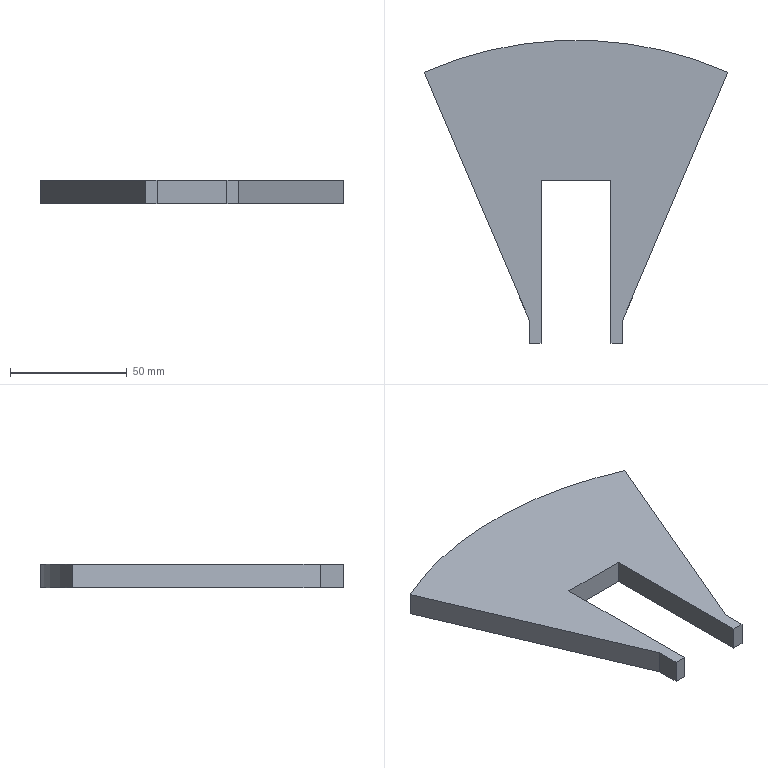Part | SolidWorks | features Extrusion 1 | 1 solid | 12 faces | box 130.202 x 130 x 10 mm | volume 85461 mm3 | plane 11 | cylinder 1 | commonest cylinder face diameters 322 x1
STEP:
#1=CARTESIAN_POINT('',(20.,41.,-5.));
#2=VERTEX_POINT('',#1);
#3=CARTESIAN_POINT('',(65.101,147.251,-5.));
#4=VERTEX_POINT('',#3);
#5=CARTESIAN_POINT('',(2.2,-0.9339,-5.));
#6=DIRECTION('',(0.3907,0.9205,0.));
#7=VECTOR('',#6,1000.);
#8=LINE('',#5,#7);
#9=EDGE_CURVE('',#2,#4,#8,.T.);
#10=ORIENTED_EDGE('',*,*,#9,.T.);
#11=CARTESIAN_POINT('',(65.101,147.251,5.));
#12=VERTEX_POINT('',#11);
#13=CARTESIAN_POINT('',(65.101,147.251,5.));
#14=DIRECTION('',(0.,0.,-1.));
#15=VECTOR('',#14,1000.);
#16=LINE('',#13,#15);
#17=EDGE_CURVE('',#12,#4,#16,.T.);
#18=ORIENTED_EDGE('',*,*,#17,.F.);
#19=CARTESIAN_POINT('',(20.,41.,5.));
#20=VERTEX_POINT('',#19);
#21=CARTESIAN_POINT('',(2.2,-0.9339,5.));
#22=DIRECTION('',(0.3907,0.9205,0.));
#23=VECTOR('',#22,1000.);
#24=LINE('',#21,#23);
#25=EDGE_CURVE('',#20,#12,#24,.T.);
#26=ORIENTED_EDGE('',*,*,#25,.F.);
#27=CARTESIAN_POINT('',(20.,41.,5.));
#28=DIRECTION('',(0.,0.,-1.));
#29=VECTOR('',#28,1000.);
#30=LINE('',#27,#29);
#31=EDGE_CURVE('',#20,#2,#30,.T.);
#32=ORIENTED_EDGE('',*,*,#31,.T.);
#33=EDGE_LOOP('',(#10,#18,#26,#32));
#34=FACE_OUTER_BOUND('',#33,.T.);
#35=CARTESIAN_POINT('',(2.2,-0.9339,5.));
#36=DIRECTION('',(-0.9205,0.3907,0.));
#37=DIRECTION('',(-0.3907,-0.9205,0.));
#38=AXIS2_PLACEMENT_3D('',#35,#36,#37);
#39=PLANE('',#38);
#40=ADVANCED_FACE('',(#34),#39,.F.);
#41=CARTESIAN_POINT('',(-65.101,147.251,-5.));
#42=VERTEX_POINT('',#41);
#43=CARTESIAN_POINT('',(0.,0.,-5.));
#44=DIRECTION('',(0.,0.,1.));
#45=DIRECTION('',(1.,0.,0.));
#46=AXIS2_PLACEMENT_3D('',#43,#44,#45);
#47=CIRCLE('',#46,161.);
#48=EDGE_CURVE('',#4,#42,#47,.T.);
#49=ORIENTED_EDGE('',*,*,#48,.T.);
#50=CARTESIAN_POINT('',(-65.101,147.251,5.));
#51=VERTEX_POINT('',#50);
#52=CARTESIAN_POINT('',(-65.101,147.251,5.));
#53=DIRECTION('',(0.,0.,-1.));
#54=VECTOR('',#53,1000.);
#55=LINE('',#52,#54);
#56=EDGE_CURVE('',#51,#42,#55,.T.);
#57=ORIENTED_EDGE('',*,*,#56,.F.);
#58=CARTESIAN_POINT('',(0.,0.,5.));
#59=DIRECTION('',(0.,0.,1.));
#60=DIRECTION('',(1.,0.,0.));
#61=AXIS2_PLACEMENT_3D('',#58,#59,#60);
#62=CIRCLE('',#61,161.);
#63=EDGE_CURVE('',#12,#51,#62,.T.);
#64=ORIENTED_EDGE('',*,*,#63,.F.);
#65=ORIENTED_EDGE('',*,*,#17,.T.);
#66=EDGE_LOOP('',(#49,#57,#64,#65));
#67=FACE_OUTER_BOUND('',#66,.T.);
#68=CARTESIAN_POINT('',(0.,0.,5.));
#69=DIRECTION('',(0.,0.,-1.));
#70=DIRECTION('',(-1.,0.,0.));
#71=AXIS2_PLACEMENT_3D('',#68,#69,#70);
#72=CYLINDRICAL_SURFACE('',#71,161.);
#73=ADVANCED_FACE('',(#67),#72,.T.);
#74=CARTESIAN_POINT('',(-20.,41.,-5.));
#75=VERTEX_POINT('',#74);
#76=CARTESIAN_POINT('',(-2.2,-0.9339,-5.));
#77=DIRECTION('',(0.3907,-0.9205,0.));
#78=VECTOR('',#77,1000.);
#79=LINE('',#76,#78);
#80=EDGE_CURVE('',#42,#75,#79,.T.);
#81=ORIENTED_EDGE('',*,*,#80,.T.);
#82=CARTESIAN_POINT('',(-20.,41.,5.));
#83=VERTEX_POINT('',#82);
#84=CARTESIAN_POINT('',(-20.,41.,5.));
#85=DIRECTION('',(0.,0.,-1.));
#86=VECTOR('',#85,1000.);
#87=LINE('',#84,#86);
#88=EDGE_CURVE('',#83,#75,#87,.T.);
#89=ORIENTED_EDGE('',*,*,#88,.F.);
#90=CARTESIAN_POINT('',(-2.2,-0.9339,5.));
#91=DIRECTION('',(0.3907,-0.9205,0.));
#92=VECTOR('',#91,1000.);
#93=LINE('',#90,#92);
#94=EDGE_CURVE('',#51,#83,#93,.T.);
#95=ORIENTED_EDGE('',*,*,#94,.F.);
#96=ORIENTED_EDGE('',*,*,#56,.T.);
#97=EDGE_LOOP('',(#81,#89,#95,#96));
#98=FACE_OUTER_BOUND('',#97,.T.);
#99=CARTESIAN_POINT('',(-2.2,-0.9339,5.));
#100=DIRECTION('',(0.9205,0.3907,0.));
#101=DIRECTION('',(-0.3907,0.9205,0.));
#102=AXIS2_PLACEMENT_3D('',#99,#100,#101);
#103=PLANE('',#102);
#104=ADVANCED_FACE('',(#98),#103,.F.);
#105=CARTESIAN_POINT('',(-20.,31.,-5.));
#106=VERTEX_POINT('',#105);
#107=CARTESIAN_POINT('',(-20.,0.,-5.));
#108=DIRECTION('',(0.,-1.,0.));
#109=VECTOR('',#108,1000.);
#110=LINE('',#107,#109);
#111=EDGE_CURVE('',#75,#106,#110,.T.);
#112=ORIENTED_EDGE('',*,*,#111,.T.);
#113=CARTESIAN_POINT('',(-20.,31.,5.));
#114=VERTEX_POINT('',#113);
#115=CARTESIAN_POINT('',(-20.,31.,5.));
#116=DIRECTION('',(0.,0.,-1.));
#117=VECTOR('',#116,1000.);
#118=LINE('',#115,#117);
#119=EDGE_CURVE('',#114,#106,#118,.T.);
#120=ORIENTED_EDGE('',*,*,#119,.F.);
#121=CARTESIAN_POINT('',(-20.,0.,5.));
#122=DIRECTION('',(0.,-1.,0.));
#123=VECTOR('',#122,1000.);
#124=LINE('',#121,#123);
#125=EDGE_CURVE('',#83,#114,#124,.T.);
#126=ORIENTED_EDGE('',*,*,#125,.F.);
#127=ORIENTED_EDGE('',*,*,#88,.T.);
#128=EDGE_LOOP('',(#112,#120,#126,#127));
#129=FACE_OUTER_BOUND('',#128,.T.);
#130=CARTESIAN_POINT('',(-20.,0.,5.));
#131=DIRECTION('',(1.,0.,0.));
#132=DIRECTION('',(0.,1.,0.));
#133=AXIS2_PLACEMENT_3D('',#130,#131,#132);
#134=PLANE('',#133);
#135=ADVANCED_FACE('',(#129),#134,.F.);
#136=CARTESIAN_POINT('',(-15.,31.,-5.));
#137=VERTEX_POINT('',#136);
#138=CARTESIAN_POINT('',(0.,31.,-5.));
#139=DIRECTION('',(1.,0.,0.));
#140=VECTOR('',#139,1000.);
#141=LINE('',#138,#140);
#142=EDGE_CURVE('',#106,#137,#141,.T.);
#143=ORIENTED_EDGE('',*,*,#142,.T.);
#144=CARTESIAN_POINT('',(-15.,31.,5.));
#145=VERTEX_POINT('',#144);
#146=CARTESIAN_POINT('',(-15.,31.,5.));
#147=DIRECTION('',(0.,0.,-1.));
#148=VECTOR('',#147,1000.);
#149=LINE('',#146,#148);
#150=EDGE_CURVE('',#145,#137,#149,.T.);
#151=ORIENTED_EDGE('',*,*,#150,.F.);
#152=CARTESIAN_POINT('',(0.,31.,5.));
#153=DIRECTION('',(1.,0.,0.));
#154=VECTOR('',#153,1000.);
#155=LINE('',#152,#154);
#156=EDGE_CURVE('',#114,#145,#155,.T.);
#157=ORIENTED_EDGE('',*,*,#156,.F.);
#158=ORIENTED_EDGE('',*,*,#119,.T.);
#159=EDGE_LOOP('',(#143,#151,#157,#158));
#160=FACE_OUTER_BOUND('',#159,.T.);
#161=CARTESIAN_POINT('',(0.,31.,5.));
#162=DIRECTION('',(0.,1.,0.));
#163=DIRECTION('',(-1.,0.,0.));
#164=AXIS2_PLACEMENT_3D('',#161,#162,#163);
#165=PLANE('',#164);
#166=ADVANCED_FACE('',(#160),#165,.F.);
#167=CARTESIAN_POINT('',(-15.,101.,-5.));
#168=VERTEX_POINT('',#167);
#169=CARTESIAN_POINT('',(-15.,0.,-5.));
#170=DIRECTION('',(0.,1.,0.));
#171=VECTOR('',#170,1000.);
#172=LINE('',#169,#171);
#173=EDGE_CURVE('',#137,#168,#172,.T.);
#174=ORIENTED_EDGE('',*,*,#173,.T.);
#175=CARTESIAN_POINT('',(-15.,101.,5.));
#176=VERTEX_POINT('',#175);
#177=CARTESIAN_POINT('',(-15.,101.,5.));
#178=DIRECTION('',(0.,0.,-1.));
#179=VECTOR('',#178,1000.);
#180=LINE('',#177,#179);
#181=EDGE_CURVE('',#176,#168,#180,.T.);
#182=ORIENTED_EDGE('',*,*,#181,.F.);
#183=CARTESIAN_POINT('',(-15.,0.,5.));
#184=DIRECTION('',(0.,1.,0.));
#185=VECTOR('',#184,1000.);
#186=LINE('',#183,#185);
#187=EDGE_CURVE('',#145,#176,#186,.T.);
#188=ORIENTED_EDGE('',*,*,#187,.F.);
#189=ORIENTED_EDGE('',*,*,#150,.T.);
#190=EDGE_LOOP('',(#174,#182,#188,#189));
#191=FACE_OUTER_BOUND('',#190,.T.);
#192=CARTESIAN_POINT('',(-15.,0.,5.));
#193=DIRECTION('',(-1.,0.,0.));
#194=DIRECTION('',(0.,0.,1.));
#195=AXIS2_PLACEMENT_3D('',#192,#193,#194);
#196=PLANE('',#195);
#197=ADVANCED_FACE('',(#191),#196,.F.);
#198=CARTESIAN_POINT('',(15.,101.,-5.));
#199=VERTEX_POINT('',#198);
#200=CARTESIAN_POINT('',(0.,101.,-5.));
#201=DIRECTION('',(-1.,0.,0.));
#202=VECTOR('',#201,1000.);
#203=LINE('',#200,#202);
#204=EDGE_CURVE('',#199,#168,#203,.T.);
#205=ORIENTED_EDGE('',*,*,#204,.F.);
#206=CARTESIAN_POINT('',(15.,101.,5.));
#207=VERTEX_POINT('',#206);
#208=CARTESIAN_POINT('',(15.,101.,5.));
#209=DIRECTION('',(0.,0.,-1.));
#210=VECTOR('',#209,1000.);
#211=LINE('',#208,#210);
#212=EDGE_CURVE('',#207,#199,#211,.T.);
#213=ORIENTED_EDGE('',*,*,#212,.F.);
#214=CARTESIAN_POINT('',(0.,101.,5.));
#215=DIRECTION('',(-1.,0.,0.));
#216=VECTOR('',#215,1000.);
#217=LINE('',#214,#216);
#218=EDGE_CURVE('',#207,#176,#217,.T.);
#219=ORIENTED_EDGE('',*,*,#218,.T.);
#220=ORIENTED_EDGE('',*,*,#181,.T.);
#221=EDGE_LOOP('',(#205,#213,#219,#220));
#222=FACE_OUTER_BOUND('',#221,.T.);
#223=CARTESIAN_POINT('',(0.,101.,5.));
#224=DIRECTION('',(0.,-1.,0.));
#225=DIRECTION('',(0.,0.,-1.));
#226=AXIS2_PLACEMENT_3D('',#223,#224,#225);
#227=PLANE('',#226);
#228=ADVANCED_FACE('',(#222),#227,.T.);
#229=CARTESIAN_POINT('',(15.,31.,-5.));
#230=VERTEX_POINT('',#229);
#231=CARTESIAN_POINT('',(15.,0.,-5.));
#232=DIRECTION('',(0.,1.,0.));
#233=VECTOR('',#232,1000.);
#234=LINE('',#231,#233);
#235=EDGE_CURVE('',#230,#199,#234,.T.);
#236=ORIENTED_EDGE('',*,*,#235,.F.);
#237=CARTESIAN_POINT('',(15.,31.,5.));
#238=VERTEX_POINT('',#237);
#239=CARTESIAN_POINT('',(15.,31.,5.));
#240=DIRECTION('',(0.,0.,-1.));
#241=VECTOR('',#240,1000.);
#242=LINE('',#239,#241);
#243=EDGE_CURVE('',#238,#230,#242,.T.);
#244=ORIENTED_EDGE('',*,*,#243,.F.);
#245=CARTESIAN_POINT('',(15.,0.,5.));
#246=DIRECTION('',(0.,1.,0.));
#247=VECTOR('',#246,1000.);
#248=LINE('',#245,#247);
#249=EDGE_CURVE('',#238,#207,#248,.T.);
#250=ORIENTED_EDGE('',*,*,#249,.T.);
#251=ORIENTED_EDGE('',*,*,#212,.T.);
#252=EDGE_LOOP('',(#236,#244,#250,#251));
#253=FACE_OUTER_BOUND('',#252,.T.);
#254=CARTESIAN_POINT('',(15.,0.,5.));
#255=DIRECTION('',(-1.,0.,0.));
#256=DIRECTION('',(0.,-1.,0.));
#257=AXIS2_PLACEMENT_3D('',#254,#255,#256);
#258=PLANE('',#257);
#259=ADVANCED_FACE('',(#253),#258,.T.);
#260=CARTESIAN_POINT('',(20.,31.,-5.));
#261=VERTEX_POINT('',#260);
#262=CARTESIAN_POINT('',(0.,31.,-5.));
#263=DIRECTION('',(1.,0.,0.));
#264=VECTOR('',#263,1000.);
#265=LINE('',#262,#264);
#266=EDGE_CURVE('',#230,#261,#265,.T.);
#267=ORIENTED_EDGE('',*,*,#266,.T.);
#268=CARTESIAN_POINT('',(20.,31.,5.));
#269=VERTEX_POINT('',#268);
#270=CARTESIAN_POINT('',(20.,31.,5.));
#271=DIRECTION('',(0.,0.,-1.));
#272=VECTOR('',#271,1000.);
#273=LINE('',#270,#272);
#274=EDGE_CURVE('',#269,#261,#273,.T.);
#275=ORIENTED_EDGE('',*,*,#274,.F.);
#276=CARTESIAN_POINT('',(0.,31.,5.));
#277=DIRECTION('',(1.,0.,0.));
#278=VECTOR('',#277,1000.);
#279=LINE('',#276,#278);
#280=EDGE_CURVE('',#238,#269,#279,.T.);
#281=ORIENTED_EDGE('',*,*,#280,.F.);
#282=ORIENTED_EDGE('',*,*,#243,.T.);
#283=EDGE_LOOP('',(#267,#275,#281,#282));
#284=FACE_OUTER_BOUND('',#283,.T.);
#285=CARTESIAN_POINT('',(0.,31.,5.));
#286=DIRECTION('',(0.,1.,0.));
#287=DIRECTION('',(-1.,0.,0.));
#288=AXIS2_PLACEMENT_3D('',#285,#286,#287);
#289=PLANE('',#288);
#290=ADVANCED_FACE('',(#284),#289,.F.);
#291=CARTESIAN_POINT('',(20.,0.,-5.));
#292=DIRECTION('',(0.,1.,0.));
#293=VECTOR('',#292,1000.);
#294=LINE('',#291,#293);
#295=EDGE_CURVE('',#261,#2,#294,.T.);
#296=ORIENTED_EDGE('',*,*,#295,.T.);
#297=ORIENTED_EDGE('',*,*,#31,.F.);
#298=CARTESIAN_POINT('',(20.,0.,5.));
#299=DIRECTION('',(0.,1.,0.));
#300=VECTOR('',#299,1000.);
#301=LINE('',#298,#300);
#302=EDGE_CURVE('',#269,#20,#301,.T.);
#303=ORIENTED_EDGE('',*,*,#302,.F.);
#304=ORIENTED_EDGE('',*,*,#274,.T.);
#305=EDGE_LOOP('',(#296,#297,#303,#304));
#306=FACE_OUTER_BOUND('',#305,.T.);
#307=CARTESIAN_POINT('',(20.,0.,5.));
#308=DIRECTION('',(-1.,0.,0.));
#309=DIRECTION('',(0.,-1.,0.));
#310=AXIS2_PLACEMENT_3D('',#307,#308,#309);
#311=PLANE('',#310);
#312=ADVANCED_FACE('',(#306),#311,.F.);
#313=ORIENTED_EDGE('',*,*,#25,.T.);
#314=ORIENTED_EDGE('',*,*,#63,.T.);
#315=ORIENTED_EDGE('',*,*,#94,.T.);
#316=ORIENTED_EDGE('',*,*,#125,.T.);
#317=ORIENTED_EDGE('',*,*,#156,.T.);
#318=ORIENTED_EDGE('',*,*,#187,.T.);
#319=ORIENTED_EDGE('',*,*,#218,.F.);
#320=ORIENTED_EDGE('',*,*,#249,.F.);
#321=ORIENTED_EDGE('',*,*,#280,.T.);
#322=ORIENTED_EDGE('',*,*,#302,.T.);
#323=EDGE_LOOP('',(#313,#314,#315,#316,#317,#318,#319,#320,#321,#322));
#324=FACE_OUTER_BOUND('',#323,.T.);
#325=CARTESIAN_POINT('',(0.,0.,5.));
#326=DIRECTION('',(0.,0.,1.));
#327=DIRECTION('',(1.,0.,0.));
#328=AXIS2_PLACEMENT_3D('',#325,#326,#327);
#329=PLANE('',#328);
#330=ADVANCED_FACE('',(#324),#329,.T.);
#331=ORIENTED_EDGE('',*,*,#9,.F.);
#332=ORIENTED_EDGE('',*,*,#295,.F.);
#333=ORIENTED_EDGE('',*,*,#266,.F.);
#334=ORIENTED_EDGE('',*,*,#235,.T.);
#335=ORIENTED_EDGE('',*,*,#204,.T.);
#336=ORIENTED_EDGE('',*,*,#173,.F.);
#337=ORIENTED_EDGE('',*,*,#142,.F.);
#338=ORIENTED_EDGE('',*,*,#111,.F.);
#339=ORIENTED_EDGE('',*,*,#80,.F.);
#340=ORIENTED_EDGE('',*,*,#48,.F.);
#341=EDGE_LOOP('',(#331,#332,#333,#334,#335,#336,#337,#338,#339,#340));
#342=FACE_OUTER_BOUND('',#341,.T.);
#343=CARTESIAN_POINT('',(0.,0.,-5.));
#344=DIRECTION('',(0.,0.,1.));
#345=DIRECTION('',(1.,0.,0.));
#346=AXIS2_PLACEMENT_3D('',#343,#344,#345);
#347=PLANE('',#346);
#348=ADVANCED_FACE('',(#342),#347,.F.);
#349=CLOSED_SHELL('',(#40,#73,#104,#135,#166,#197,#228,#259,#290,#312,#330,#348));
#350=MANIFOLD_SOLID_BREP('',#349);
#351=CARTESIAN_POINT('',(0.,0.,0.));
#352=DIRECTION('',(0.,0.,1.));
#353=DIRECTION('',(1.,0.,0.));
#354=AXIS2_PLACEMENT_3D('',#351,#352,#353);
#355=(LENGTH_UNIT()NAMED_UNIT(*)SI_UNIT(.MILLI.,.METRE.));
#356=UNCERTAINTY_MEASURE_WITH_UNIT(LENGTH_MEASURE(0.00001),#355,'','');
#357=(NAMED_UNIT(*)PLANE_ANGLE_UNIT()SI_UNIT($,.RADIAN.));
#358=(NAMED_UNIT(*)SI_UNIT($,.STERADIAN.)SOLID_ANGLE_UNIT());
#359=(GEOMETRIC_REPRESENTATION_CONTEXT(3)GLOBAL_UNCERTAINTY_ASSIGNED_CONTEXT((#356))GLOBAL_UNIT_ASSIGNED_CONTEXT((#355,#357,#358))REPRESENTATION_CONTEXT('',''));
#360=ADVANCED_BREP_SHAPE_REPRESENTATION('',(#350,#354),#359);